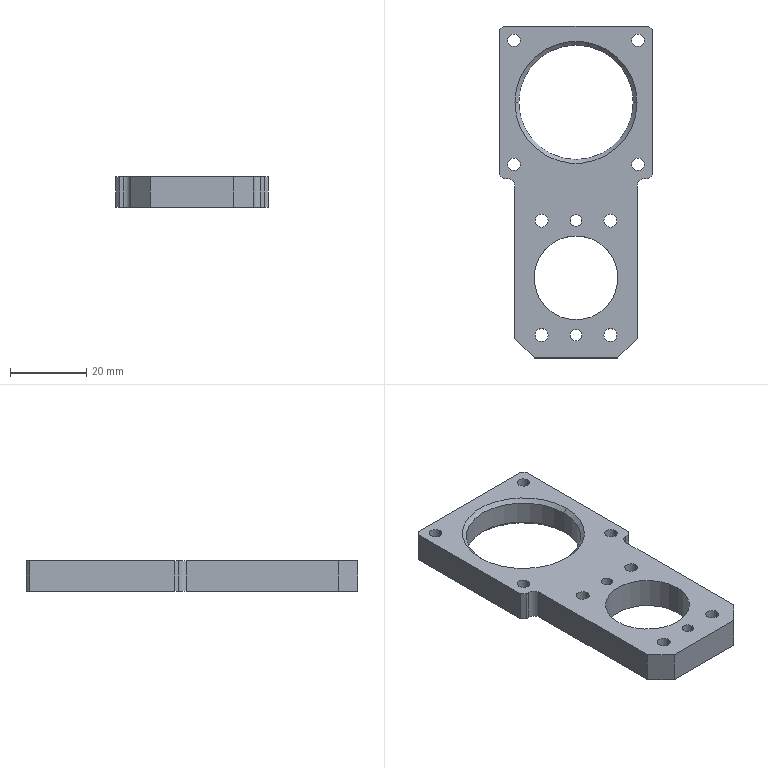Part | SolidWorks | features Chamfer 2, HoleWzd 2, Extrusion 1, Fillet 1, ICE 1 | 1 solid | 46 faces | box 40 x 87 x 8 mm | volume 15160 mm3 | cylinder 26 | plane 16 | cone 4 | commonest cylinder face diameters 3.3 x8 3.4 x8 3 x4 4 x2 22 x2 30 x2
STEP:
#1=CARTESIAN_POINT('',(-15.,23.5,3.));
#2=VERTEX_POINT('',#1);
#3=CARTESIAN_POINT('',(15.,23.5,3.));
#4=VERTEX_POINT('',#3);
#5=CARTESIAN_POINT('',(0.,23.5,3.));
#6=DIRECTION('',(0.,0.,1.));
#7=DIRECTION('',(1.,0.,0.));
#8=AXIS2_PLACEMENT_3D('',#5,#6,#7);
#9=CIRCLE('',#8,15.);
#10=EDGE_CURVE('',#2,#4,#9,.T.);
#11=ORIENTED_EDGE('',*,*,#10,.F.);
#12=CARTESIAN_POINT('',(-16.,23.5,4.));
#13=VERTEX_POINT('',#12);
#14=CARTESIAN_POINT('',(-15.,23.5,3.));
#15=DIRECTION('',(-0.7071,0.,0.7071));
#16=VECTOR('',#15,1000.);
#17=LINE('',#14,#16);
#18=EDGE_CURVE('',#2,#13,#17,.T.);
#19=ORIENTED_EDGE('',*,*,#18,.T.);
#20=CARTESIAN_POINT('',(16.,23.5,4.));
#21=VERTEX_POINT('',#20);
#22=CARTESIAN_POINT('',(0.,23.5,4.));
#23=DIRECTION('',(0.,0.,-1.));
#24=DIRECTION('',(1.,0.,0.));
#25=AXIS2_PLACEMENT_3D('',#22,#23,#24);
#26=CIRCLE('',#25,16.);
#27=EDGE_CURVE('',#21,#13,#26,.T.);
#28=ORIENTED_EDGE('',*,*,#27,.F.);
#29=CARTESIAN_POINT('',(15.,23.5,3.));
#30=DIRECTION('',(0.7071,0.,0.7071));
#31=VECTOR('',#30,1000.);
#32=LINE('',#29,#31);
#33=EDGE_CURVE('',#4,#21,#32,.T.);
#34=ORIENTED_EDGE('',*,*,#33,.F.);
#35=EDGE_LOOP('',(#11,#19,#28,#34));
#36=FACE_OUTER_BOUND('',#35,.T.);
#37=CARTESIAN_POINT('',(0.,23.5,3.));
#38=DIRECTION('',(0.,0.,1.));
#39=DIRECTION('',(1.,0.,0.));
#40=AXIS2_PLACEMENT_3D('',#37,#38,#39);
#41=CONICAL_SURFACE('',#40,15.,0.7854);
#42=ADVANCED_FACE('',(#36),#41,.F.);
#43=CARTESIAN_POINT('',(15.,23.5,-3.));
#44=VERTEX_POINT('',#43);
#45=CARTESIAN_POINT('',(-15.,23.5,-3.));
#46=VERTEX_POINT('',#45);
#47=CARTESIAN_POINT('',(0.,23.5,-3.));
#48=DIRECTION('',(0.,0.,-1.));
#49=DIRECTION('',(1.,0.,0.));
#50=AXIS2_PLACEMENT_3D('',#47,#48,#49);
#51=CIRCLE('',#50,15.);
#52=EDGE_CURVE('',#44,#46,#51,.T.);
#53=ORIENTED_EDGE('',*,*,#52,.F.);
#54=CARTESIAN_POINT('',(16.,23.5,-4.));
#55=VERTEX_POINT('',#54);
#56=CARTESIAN_POINT('',(16.,23.5,-4.));
#57=DIRECTION('',(0.7071,0.,-0.7071));
#58=VECTOR('',#57,1000.);
#59=LINE('',#56,#58);
#60=EDGE_CURVE('',#44,#55,#59,.T.);
#61=ORIENTED_EDGE('',*,*,#60,.T.);
#62=CARTESIAN_POINT('',(-16.,23.5,-4.));
#63=VERTEX_POINT('',#62);
#64=CARTESIAN_POINT('',(0.,23.5,-4.));
#65=DIRECTION('',(0.,0.,1.));
#66=DIRECTION('',(1.,0.,0.));
#67=AXIS2_PLACEMENT_3D('',#64,#65,#66);
#68=CIRCLE('',#67,16.);
#69=EDGE_CURVE('',#63,#55,#68,.T.);
#70=ORIENTED_EDGE('',*,*,#69,.F.);
#71=CARTESIAN_POINT('',(-16.,23.5,-4.));
#72=DIRECTION('',(-0.7071,0.,-0.7071));
#73=VECTOR('',#72,1000.);
#74=LINE('',#71,#73);
#75=EDGE_CURVE('',#46,#63,#74,.T.);
#76=ORIENTED_EDGE('',*,*,#75,.F.);
#77=EDGE_LOOP('',(#53,#61,#70,#76));
#78=FACE_OUTER_BOUND('',#77,.T.);
#79=CARTESIAN_POINT('',(0.,23.5,-4.));
#80=DIRECTION('',(0.,0.,-1.));
#81=DIRECTION('',(-1.,0.,0.));
#82=AXIS2_PLACEMENT_3D('',#79,#80,#81);
#83=CONICAL_SURFACE('',#82,16.,0.7854);
#84=ADVANCED_FACE('',(#78),#83,.F.);
#85=CARTESIAN_POINT('',(-11.,-22.5,-4.));
#86=VERTEX_POINT('',#85);
#87=CARTESIAN_POINT('',(11.,-22.5,-4.));
#88=VERTEX_POINT('',#87);
#89=CARTESIAN_POINT('',(0.,-22.5,-4.));
#90=DIRECTION('',(0.,0.,1.));
#91=DIRECTION('',(1.,0.,0.));
#92=AXIS2_PLACEMENT_3D('',#89,#90,#91);
#93=CIRCLE('',#92,11.);
#94=EDGE_CURVE('',#86,#88,#93,.T.);
#95=ORIENTED_EDGE('',*,*,#94,.F.);
#96=CARTESIAN_POINT('',(-11.,-22.5,4.));
#97=VERTEX_POINT('',#96);
#98=CARTESIAN_POINT('',(-11.,-22.5,-4.));
#99=DIRECTION('',(0.,0.,1.));
#100=VECTOR('',#99,1000.);
#101=LINE('',#98,#100);
#102=EDGE_CURVE('',#86,#97,#101,.T.);
#103=ORIENTED_EDGE('',*,*,#102,.T.);
#104=CARTESIAN_POINT('',(11.,-22.5,4.));
#105=VERTEX_POINT('',#104);
#106=CARTESIAN_POINT('',(0.,-22.5,4.));
#107=DIRECTION('',(0.,0.,1.));
#108=DIRECTION('',(1.,0.,0.));
#109=AXIS2_PLACEMENT_3D('',#106,#107,#108);
#110=CIRCLE('',#109,11.);
#111=EDGE_CURVE('',#97,#105,#110,.T.);
#112=ORIENTED_EDGE('',*,*,#111,.T.);
#113=CARTESIAN_POINT('',(11.,-22.5,-4.));
#114=DIRECTION('',(0.,0.,1.));
#115=VECTOR('',#114,1000.);
#116=LINE('',#113,#115);
#117=EDGE_CURVE('',#88,#105,#116,.T.);
#118=ORIENTED_EDGE('',*,*,#117,.F.);
#119=EDGE_LOOP('',(#95,#103,#112,#118));
#120=FACE_OUTER_BOUND('',#119,.T.);
#121=CARTESIAN_POINT('',(0.,-22.5,-4.));
#122=DIRECTION('',(0.,0.,1.));
#123=DIRECTION('',(1.,0.,0.));
#124=AXIS2_PLACEMENT_3D('',#121,#122,#123);
#125=CYLINDRICAL_SURFACE('',#124,11.);
#126=ADVANCED_FACE('',(#120),#125,.F.);
#127=CARTESIAN_POINT('',(-1.5,-37.5,-4.));
#128=VERTEX_POINT('',#127);
#129=CARTESIAN_POINT('',(1.5,-37.5,-4.));
#130=VERTEX_POINT('',#129);
#131=CARTESIAN_POINT('',(0.,-37.5,-4.));
#132=DIRECTION('',(0.,0.,1.));
#133=DIRECTION('',(1.,0.,0.));
#134=AXIS2_PLACEMENT_3D('',#131,#132,#133);
#135=CIRCLE('',#134,1.5);
#136=EDGE_CURVE('',#128,#130,#135,.T.);
#137=ORIENTED_EDGE('',*,*,#136,.F.);
#138=CARTESIAN_POINT('',(-1.5,-37.5,4.));
#139=VERTEX_POINT('',#138);
#140=CARTESIAN_POINT('',(-1.5,-37.5,-4.));
#141=DIRECTION('',(0.,0.,1.));
#142=VECTOR('',#141,1000.);
#143=LINE('',#140,#142);
#144=EDGE_CURVE('',#128,#139,#143,.T.);
#145=ORIENTED_EDGE('',*,*,#144,.T.);
#146=CARTESIAN_POINT('',(1.5,-37.5,4.));
#147=VERTEX_POINT('',#146);
#148=CARTESIAN_POINT('',(0.,-37.5,4.));
#149=DIRECTION('',(0.,0.,1.));
#150=DIRECTION('',(1.,0.,0.));
#151=AXIS2_PLACEMENT_3D('',#148,#149,#150);
#152=CIRCLE('',#151,1.5);
#153=EDGE_CURVE('',#139,#147,#152,.T.);
#154=ORIENTED_EDGE('',*,*,#153,.T.);
#155=CARTESIAN_POINT('',(1.5,-37.5,-4.));
#156=DIRECTION('',(0.,0.,1.));
#157=VECTOR('',#156,1000.);
#158=LINE('',#155,#157);
#159=EDGE_CURVE('',#130,#147,#158,.T.);
#160=ORIENTED_EDGE('',*,*,#159,.F.);
#161=EDGE_LOOP('',(#137,#145,#154,#160));
#162=FACE_OUTER_BOUND('',#161,.T.);
#163=CARTESIAN_POINT('',(0.,-37.5,-4.));
#164=DIRECTION('',(0.,0.,1.));
#165=DIRECTION('',(1.,0.,0.));
#166=AXIS2_PLACEMENT_3D('',#163,#164,#165);
#167=CYLINDRICAL_SURFACE('',#166,1.5);
#168=ADVANCED_FACE('',(#162),#167,.F.);
#169=CARTESIAN_POINT('',(-1.5,-7.5,-4.));
#170=VERTEX_POINT('',#169);
#171=CARTESIAN_POINT('',(1.5,-7.5,-4.));
#172=VERTEX_POINT('',#171);
#173=CARTESIAN_POINT('',(0.,-7.5,-4.));
#174=DIRECTION('',(0.,0.,1.));
#175=DIRECTION('',(1.,0.,0.));
#176=AXIS2_PLACEMENT_3D('',#173,#174,#175);
#177=CIRCLE('',#176,1.5);
#178=EDGE_CURVE('',#170,#172,#177,.T.);
#179=ORIENTED_EDGE('',*,*,#178,.F.);
#180=CARTESIAN_POINT('',(-1.5,-7.5,4.));
#181=VERTEX_POINT('',#180);
#182=CARTESIAN_POINT('',(-1.5,-7.5,-4.));
#183=DIRECTION('',(0.,0.,1.));
#184=VECTOR('',#183,1000.);
#185=LINE('',#182,#184);
#186=EDGE_CURVE('',#170,#181,#185,.T.);
#187=ORIENTED_EDGE('',*,*,#186,.T.);
#188=CARTESIAN_POINT('',(1.5,-7.5,4.));
#189=VERTEX_POINT('',#188);
#190=CARTESIAN_POINT('',(0.,-7.5,4.));
#191=DIRECTION('',(0.,0.,1.));
#192=DIRECTION('',(1.,0.,0.));
#193=AXIS2_PLACEMENT_3D('',#190,#191,#192);
#194=CIRCLE('',#193,1.5);
#195=EDGE_CURVE('',#181,#189,#194,.T.);
#196=ORIENTED_EDGE('',*,*,#195,.T.);
#197=CARTESIAN_POINT('',(1.5,-7.5,-4.));
#198=DIRECTION('',(0.,0.,1.));
#199=VECTOR('',#198,1000.);
#200=LINE('',#197,#199);
#201=EDGE_CURVE('',#172,#189,#200,.T.);
#202=ORIENTED_EDGE('',*,*,#201,.F.);
#203=EDGE_LOOP('',(#179,#187,#196,#202));
#204=FACE_OUTER_BOUND('',#203,.T.);
#205=CARTESIAN_POINT('',(0.,-7.5,-4.));
#206=DIRECTION('',(0.,0.,1.));
#207=DIRECTION('',(1.,0.,0.));
#208=AXIS2_PLACEMENT_3D('',#205,#206,#207);
#209=CYLINDRICAL_SURFACE('',#208,1.5);
#210=ADVANCED_FACE('',(#204),#209,.F.);
#211=ORIENTED_EDGE('',*,*,#52,.T.);
#212=CARTESIAN_POINT('',(-15.,23.5,-4.));
#213=DIRECTION('',(0.,0.,1.));
#214=VECTOR('',#213,1000.);
#215=LINE('',#212,#214);
#216=EDGE_CURVE('',#46,#2,#215,.T.);
#217=ORIENTED_EDGE('',*,*,#216,.T.);
#218=ORIENTED_EDGE('',*,*,#10,.T.);
#219=CARTESIAN_POINT('',(15.,23.5,-4.));
#220=DIRECTION('',(0.,0.,1.));
#221=VECTOR('',#220,1000.);
#222=LINE('',#219,#221);
#223=EDGE_CURVE('',#44,#4,#222,.T.);
#224=ORIENTED_EDGE('',*,*,#223,.F.);
#225=EDGE_LOOP('',(#211,#217,#218,#224));
#226=FACE_OUTER_BOUND('',#225,.T.);
#227=CARTESIAN_POINT('',(0.,23.5,-4.));
#228=DIRECTION('',(0.,0.,1.));
#229=DIRECTION('',(1.,0.,0.));
#230=AXIS2_PLACEMENT_3D('',#227,#228,#229);
#231=CYLINDRICAL_SURFACE('',#230,15.);
#232=ADVANCED_FACE('',(#226),#231,.F.);
#233=CARTESIAN_POINT('',(-10.7,-7.5,-4.));
#234=VERTEX_POINT('',#233);
#235=CARTESIAN_POINT('',(-7.3,-7.5,-4.));
#236=VERTEX_POINT('',#235);
#237=CARTESIAN_POINT('',(-9.,-7.5,-4.));
#238=DIRECTION('',(0.,0.,1.));
#239=DIRECTION('',(1.,0.,0.));
#240=AXIS2_PLACEMENT_3D('',#237,#238,#239);
#241=CIRCLE('',#240,1.7);
#242=EDGE_CURVE('',#234,#236,#241,.T.);
#243=ORIENTED_EDGE('',*,*,#242,.F.);
#244=CARTESIAN_POINT('',(-10.7,-7.5,4.));
#245=VERTEX_POINT('',#244);
#246=CARTESIAN_POINT('',(-10.7,-7.5,4.));
#247=DIRECTION('',(0.,0.,1.));
#248=VECTOR('',#247,1000.);
#249=LINE('',#246,#248);
#250=EDGE_CURVE('',#234,#245,#249,.T.);
#251=ORIENTED_EDGE('',*,*,#250,.T.);
#252=CARTESIAN_POINT('',(-7.3,-7.5,4.));
#253=VERTEX_POINT('',#252);
#254=CARTESIAN_POINT('',(-9.,-7.5,4.));
#255=DIRECTION('',(0.,0.,1.));
#256=DIRECTION('',(1.,0.,0.));
#257=AXIS2_PLACEMENT_3D('',#254,#255,#256);
#258=CIRCLE('',#257,1.7);
#259=EDGE_CURVE('',#245,#253,#258,.T.);
#260=ORIENTED_EDGE('',*,*,#259,.T.);
#261=CARTESIAN_POINT('',(-7.3,-7.5,4.));
#262=DIRECTION('',(0.,0.,1.));
#263=VECTOR('',#262,1000.);
#264=LINE('',#261,#263);
#265=EDGE_CURVE('',#236,#253,#264,.T.);
#266=ORIENTED_EDGE('',*,*,#265,.F.);
#267=EDGE_LOOP('',(#243,#251,#260,#266));
#268=FACE_OUTER_BOUND('',#267,.T.);
#269=CARTESIAN_POINT('',(-9.,-7.5,4.));
#270=DIRECTION('',(0.,0.,1.));
#271=DIRECTION('',(1.,0.,0.));
#272=AXIS2_PLACEMENT_3D('',#269,#270,#271);
#273=CYLINDRICAL_SURFACE('',#272,1.7);
#274=ADVANCED_FACE('',(#268),#273,.F.);
#275=CARTESIAN_POINT('',(7.3,-7.5,-4.));
#276=VERTEX_POINT('',#275);
#277=CARTESIAN_POINT('',(10.7,-7.5,-4.));
#278=VERTEX_POINT('',#277);
#279=CARTESIAN_POINT('',(9.,-7.5,-4.));
#280=DIRECTION('',(0.,0.,1.));
#281=DIRECTION('',(1.,0.,0.));
#282=AXIS2_PLACEMENT_3D('',#279,#280,#281);
#283=CIRCLE('',#282,1.7);
#284=EDGE_CURVE('',#276,#278,#283,.T.);
#285=ORIENTED_EDGE('',*,*,#284,.F.);
#286=CARTESIAN_POINT('',(7.3,-7.5,4.));
#287=VERTEX_POINT('',#286);
#288=CARTESIAN_POINT('',(7.3,-7.5,4.));
#289=DIRECTION('',(0.,0.,1.));
#290=VECTOR('',#289,1000.);
#291=LINE('',#288,#290);
#292=EDGE_CURVE('',#276,#287,#291,.T.);
#293=ORIENTED_EDGE('',*,*,#292,.T.);
#294=CARTESIAN_POINT('',(10.7,-7.5,4.));
#295=VERTEX_POINT('',#294);
#296=CARTESIAN_POINT('',(9.,-7.5,4.));
#297=DIRECTION('',(0.,0.,1.));
#298=DIRECTION('',(1.,0.,0.));
#299=AXIS2_PLACEMENT_3D('',#296,#297,#298);
#300=CIRCLE('',#299,1.7);
#301=EDGE_CURVE('',#287,#295,#300,.T.);
#302=ORIENTED_EDGE('',*,*,#301,.T.);
#303=CARTESIAN_POINT('',(10.7,-7.5,4.));
#304=DIRECTION('',(0.,0.,1.));
#305=VECTOR('',#304,1000.);
#306=LINE('',#303,#305);
#307=EDGE_CURVE('',#278,#295,#306,.T.);
#308=ORIENTED_EDGE('',*,*,#307,.F.);
#309=EDGE_LOOP('',(#285,#293,#302,#308));
#310=FACE_OUTER_BOUND('',#309,.T.);
#311=CARTESIAN_POINT('',(9.,-7.5,4.));
#312=DIRECTION('',(0.,0.,1.));
#313=DIRECTION('',(1.,0.,0.));
#314=AXIS2_PLACEMENT_3D('',#311,#312,#313);
#315=CYLINDRICAL_SURFACE('',#314,1.7);
#316=ADVANCED_FACE('',(#310),#315,.F.);
#317=CARTESIAN_POINT('',(7.3,-37.5,-4.));
#318=VERTEX_POINT('',#317);
#319=CARTESIAN_POINT('',(10.7,-37.5,-4.));
#320=VERTEX_POINT('',#319);
#321=CARTESIAN_POINT('',(9.,-37.5,-4.));
#322=DIRECTION('',(0.,0.,1.));
#323=DIRECTION('',(1.,0.,0.));
#324=AXIS2_PLACEMENT_3D('',#321,#322,#323);
#325=CIRCLE('',#324,1.7);
#326=EDGE_CURVE('',#318,#320,#325,.T.);
#327=ORIENTED_EDGE('',*,*,#326,.F.);
#328=CARTESIAN_POINT('',(7.3,-37.5,4.));
#329=VERTEX_POINT('',#328);
#330=CARTESIAN_POINT('',(7.3,-37.5,4.));
#331=DIRECTION('',(0.,0.,1.));
#332=VECTOR('',#331,1000.);
#333=LINE('',#330,#332);
#334=EDGE_CURVE('',#318,#329,#333,.T.);
#335=ORIENTED_EDGE('',*,*,#334,.T.);
#336=CARTESIAN_POINT('',(10.7,-37.5,4.));
#337=VERTEX_POINT('',#336);
#338=CARTESIAN_POINT('',(9.,-37.5,4.));
#339=DIRECTION('',(0.,0.,1.));
#340=DIRECTION('',(1.,0.,0.));
#341=AXIS2_PLACEMENT_3D('',#338,#339,#340);
#342=CIRCLE('',#341,1.7);
#343=EDGE_CURVE('',#329,#337,#342,.T.);
#344=ORIENTED_EDGE('',*,*,#343,.T.);
#345=CARTESIAN_POINT('',(10.7,-37.5,4.));
#346=DIRECTION('',(0.,0.,1.));
#347=VECTOR('',#346,1000.);
#348=LINE('',#345,#347);
#349=EDGE_CURVE('',#320,#337,#348,.T.);
#350=ORIENTED_EDGE('',*,*,#349,.F.);
#351=EDGE_LOOP('',(#327,#335,#344,#350));
#352=FACE_OUTER_BOUND('',#351,.T.);
#353=CARTESIAN_POINT('',(9.,-37.5,4.));
#354=DIRECTION('',(0.,0.,1.));
#355=DIRECTION('',(1.,0.,0.));
#356=AXIS2_PLACEMENT_3D('',#353,#354,#355);
#357=CYLINDRICAL_SURFACE('',#356,1.7);
#358=ADVANCED_FACE('',(#352),#357,.F.);
#359=CARTESIAN_POINT('',(-10.7,-37.5,-4.));
#360=VERTEX_POINT('',#359);
#361=CARTESIAN_POINT('',(-7.3,-37.5,-4.));
#362=VERTEX_POINT('',#361);
#363=CARTESIAN_POINT('',(-9.,-37.5,-4.));
#364=DIRECTION('',(0.,0.,1.));
#365=DIRECTION('',(1.,0.,0.));
#366=AXIS2_PLACEMENT_3D('',#363,#364,#365);
#367=CIRCLE('',#366,1.7);
#368=EDGE_CURVE('',#360,#362,#367,.T.);
#369=ORIENTED_EDGE('',*,*,#368,.F.);
#370=CARTESIAN_POINT('',(-10.7,-37.5,4.));
#371=VERTEX_POINT('',#370);
#372=CARTESIAN_POINT('',(-10.7,-37.5,4.));
#373=DIRECTION('',(0.,0.,1.));
#374=VECTOR('',#373,1000.);
#375=LINE('',#372,#374);
#376=EDGE_CURVE('',#360,#371,#375,.T.);
#377=ORIENTED_EDGE('',*,*,#376,.T.);
#378=CARTESIAN_POINT('',(-7.3,-37.5,4.));
#379=VERTEX_POINT('',#378);
#380=CARTESIAN_POINT('',(-9.,-37.5,4.));
#381=DIRECTION('',(0.,0.,1.));
#382=DIRECTION('',(1.,0.,0.));
#383=AXIS2_PLACEMENT_3D('',#380,#381,#382);
#384=CIRCLE('',#383,1.7);
#385=EDGE_CURVE('',#371,#379,#384,.T.);
#386=ORIENTED_EDGE('',*,*,#385,.T.);
#387=CARTESIAN_POINT('',(-7.3,-37.5,4.));
#388=DIRECTION('',(0.,0.,1.));
#389=VECTOR('',#388,1000.);
#390=LINE('',#387,#389);
#391=EDGE_CURVE('',#362,#379,#390,.T.);
#392=ORIENTED_EDGE('',*,*,#391,.F.);
#393=EDGE_LOOP('',(#369,#377,#386,#392));
#394=FACE_OUTER_BOUND('',#393,.T.);
#395=CARTESIAN_POINT('',(-9.,-37.5,4.));
#396=DIRECTION('',(0.,0.,1.));
#397=DIRECTION('',(1.,0.,0.));
#398=AXIS2_PLACEMENT_3D('',#395,#396,#397);
#399=CYLINDRICAL_SURFACE('',#398,1.7);
#400=ADVANCED_FACE('',(#394),#399,.F.);
#401=CARTESIAN_POINT('',(-17.913,39.763,-4.));
#402=VERTEX_POINT('',#401);
#403=CARTESIAN_POINT('',(-14.613,39.763,-4.));
#404=VERTEX_POINT('',#403);
#405=CARTESIAN_POINT('',(-16.263,39.763,-4.));
#406=DIRECTION('',(0.,0.,1.));
#407=DIRECTION('',(1.,0.,0.));
#408=AXIS2_PLACEMENT_3D('',#405,#406,#407);
#409=CIRCLE('',#408,1.65);
#410=EDGE_CURVE('',#402,#404,#409,.T.);
#411=ORIENTED_EDGE('',*,*,#410,.F.);
#412=CARTESIAN_POINT('',(-17.913,39.763,4.));
#413=VERTEX_POINT('',#412);
#414=CARTESIAN_POINT('',(-17.913,39.763,4.));
#415=DIRECTION('',(0.,0.,1.));
#416=VECTOR('',#415,1000.);
#417=LINE('',#414,#416);
#418=EDGE_CURVE('',#402,#413,#417,.T.);
#419=ORIENTED_EDGE('',*,*,#418,.T.);
#420=CARTESIAN_POINT('',(-14.613,39.763,4.));
#421=VERTEX_POINT('',#420);
#422=CARTESIAN_POINT('',(-16.263,39.763,4.));
#423=DIRECTION('',(0.,0.,1.));
#424=DIRECTION('',(1.,0.,0.));
#425=AXIS2_PLACEMENT_3D('',#422,#423,#424);
#426=CIRCLE('',#425,1.65);
#427=EDGE_CURVE('',#413,#421,#426,.T.);
#428=ORIENTED_EDGE('',*,*,#427,.T.);
#429=CARTESIAN_POINT('',(-14.613,39.763,4.));
#430=DIRECTION('',(0.,0.,1.));
#431=VECTOR('',#430,1000.);
#432=LINE('',#429,#431);
#433=EDGE_CURVE('',#404,#421,#432,.T.);
#434=ORIENTED_EDGE('',*,*,#433,.F.);
#435=EDGE_LOOP('',(#411,#419,#428,#434));
#436=FACE_OUTER_BOUND('',#435,.T.);
#437=CARTESIAN_POINT('',(-16.263,39.763,4.));
#438=DIRECTION('',(0.,0.,1.));
#439=DIRECTION('',(1.,0.,0.));
#440=AXIS2_PLACEMENT_3D('',#437,#438,#439);
#441=CYLINDRICAL_SURFACE('',#440,1.65);
#442=ADVANCED_FACE('',(#436),#441,.F.);
#443=CARTESIAN_POINT('',(14.613,39.763,-4.));
#444=VERTEX_POINT('',#443);
#445=CARTESIAN_POINT('',(17.913,39.763,-4.));
#446=VERTEX_POINT('',#445);
#447=CARTESIAN_POINT('',(16.263,39.763,-4.));
#448=DIRECTION('',(0.,0.,1.));
#449=DIRECTION('',(1.,0.,0.));
#450=AXIS2_PLACEMENT_3D('',#447,#448,#449);
#451=CIRCLE('',#450,1.65);
#452=EDGE_CURVE('',#444,#446,#451,.T.);
#453=ORIENTED_EDGE('',*,*,#452,.F.);
#454=CARTESIAN_POINT('',(14.613,39.763,4.));
#455=VERTEX_POINT('',#454);
#456=CARTESIAN_POINT('',(14.613,39.763,4.));
#457=DIRECTION('',(0.,0.,1.));
#458=VECTOR('',#457,1000.);
#459=LINE('',#456,#458);
#460=EDGE_CURVE('',#444,#455,#459,.T.);
#461=ORIENTED_EDGE('',*,*,#460,.T.);
#462=CARTESIAN_POINT('',(17.913,39.763,4.));
#463=VERTEX_POINT('',#462);
#464=CARTESIAN_POINT('',(16.263,39.763,4.));
#465=DIRECTION('',(0.,0.,1.));
#466=DIRECTION('',(1.,0.,0.));
#467=AXIS2_PLACEMENT_3D('',#464,#465,#466);
#468=CIRCLE('',#467,1.65);
#469=EDGE_CURVE('',#455,#463,#468,.T.);
#470=ORIENTED_EDGE('',*,*,#469,.T.);
#471=CARTESIAN_POINT('',(17.913,39.763,4.));
#472=DIRECTION('',(0.,0.,1.));
#473=VECTOR('',#472,1000.);
#474=LINE('',#471,#473);
#475=EDGE_CURVE('',#446,#463,#474,.T.);
#476=ORIENTED_EDGE('',*,*,#475,.F.);
#477=EDGE_LOOP('',(#453,#461,#470,#476));
#478=FACE_OUTER_BOUND('',#477,.T.);
#479=CARTESIAN_POINT('',(16.263,39.763,4.));
#480=DIRECTION('',(0.,0.,1.));
#481=DIRECTION('',(1.,0.,0.));
#482=AXIS2_PLACEMENT_3D('',#479,#480,#481);
#483=CYLINDRICAL_SURFACE('',#482,1.65);
#484=ADVANCED_FACE('',(#478),#483,.F.);
#485=CARTESIAN_POINT('',(14.613,7.237,-4.));
#486=VERTEX_POINT('',#485);
#487=CARTESIAN_POINT('',(17.913,7.237,-4.));
#488=VERTEX_POINT('',#487);
#489=CARTESIAN_POINT('',(16.263,7.237,-4.));
#490=DIRECTION('',(0.,0.,1.));
#491=DIRECTION('',(1.,0.,0.));
#492=AXIS2_PLACEMENT_3D('',#489,#490,#491);
#493=CIRCLE('',#492,1.65);
#494=EDGE_CURVE('',#486,#488,#493,.T.);
#495=ORIENTED_EDGE('',*,*,#494,.F.);
#496=CARTESIAN_POINT('',(14.613,7.237,4.));
#497=VERTEX_POINT('',#496);
#498=CARTESIAN_POINT('',(14.613,7.237,4.));
#499=DIRECTION('',(0.,0.,1.));
#500=VECTOR('',#499,1000.);
#501=LINE('',#498,#500);
#502=EDGE_CURVE('',#486,#497,#501,.T.);
#503=ORIENTED_EDGE('',*,*,#502,.T.);
#504=CARTESIAN_POINT('',(17.913,7.237,4.));
#505=VERTEX_POINT('',#504);
#506=CARTESIAN_POINT('',(16.263,7.237,4.));
#507=DIRECTION('',(0.,0.,1.));
#508=DIRECTION('',(1.,0.,0.));
#509=AXIS2_PLACEMENT_3D('',#506,#507,#508);
#510=CIRCLE('',#509,1.65);
#511=EDGE_CURVE('',#497,#505,#510,.T.);
#512=ORIENTED_EDGE('',*,*,#511,.T.);
#513=CARTESIAN_POINT('',(17.913,7.237,4.));
#514=DIRECTION('',(0.,0.,1.));
#515=VECTOR('',#514,1000.);
#516=LINE('',#513,#515);
#517=EDGE_CURVE('',#488,#505,#516,.T.);
#518=ORIENTED_EDGE('',*,*,#517,.F.);
#519=EDGE_LOOP('',(#495,#503,#512,#518));
#520=FACE_OUTER_BOUND('',#519,.T.);
#521=CARTESIAN_POINT('',(16.263,7.237,4.));
#522=DIRECTION('',(0.,0.,1.));
#523=DIRECTION('',(1.,0.,0.));
#524=AXIS2_PLACEMENT_3D('',#521,#522,#523);
#525=CYLINDRICAL_SURFACE('',#524,1.65);
#526=ADVANCED_FACE('',(#520),#525,.F.);
#527=CARTESIAN_POINT('',(-17.913,7.237,-4.));
#528=VERTEX_POINT('',#527);
#529=CARTESIAN_POINT('',(-14.613,7.237,-4.));
#530=VERTEX_POINT('',#529);
#531=CARTESIAN_POINT('',(-16.263,7.237,-4.));
#532=DIRECTION('',(0.,0.,1.));
#533=DIRECTION('',(1.,0.,0.));
#534=AXIS2_PLACEMENT_3D('',#531,#532,#533);
#535=CIRCLE('',#534,1.65);
#536=EDGE_CURVE('',#528,#530,#535,.T.);
#537=ORIENTED_EDGE('',*,*,#536,.F.);
#538=CARTESIAN_POINT('',(-17.913,7.237,4.));
#539=VERTEX_POINT('',#538);
#540=CARTESIAN_POINT('',(-17.913,7.237,4.));
#541=DIRECTION('',(0.,0.,1.));
#542=VECTOR('',#541,1000.);
#543=LINE('',#540,#542);
#544=EDGE_CURVE('',#528,#539,#543,.T.);
#545=ORIENTED_EDGE('',*,*,#544,.T.);
#546=CARTESIAN_POINT('',(-14.613,7.237,4.));
#547=VERTEX_POINT('',#546);
#548=CARTESIAN_POINT('',(-16.263,7.237,4.));
#549=DIRECTION('',(0.,0.,1.));
#550=DIRECTION('',(1.,0.,0.));
#551=AXIS2_PLACEMENT_3D('',#548,#549,#550);
#552=CIRCLE('',#551,1.65);
#553=EDGE_CURVE('',#539,#547,#552,.T.);
#554=ORIENTED_EDGE('',*,*,#553,.T.);
#555=CARTESIAN_POINT('',(-14.613,7.237,4.));
#556=DIRECTION('',(0.,0.,1.));
#557=VECTOR('',#556,1000.);
#558=LINE('',#555,#557);
#559=EDGE_CURVE('',#530,#547,#558,.T.);
#560=ORIENTED_EDGE('',*,*,#559,.F.);
#561=EDGE_LOOP('',(#537,#545,#554,#560));
#562=FACE_OUTER_BOUND('',#561,.T.);
#563=CARTESIAN_POINT('',(-16.263,7.237,4.));
#564=DIRECTION('',(0.,0.,1.));
#565=DIRECTION('',(1.,0.,0.));
#566=AXIS2_PLACEMENT_3D('',#563,#564,#565);
#567=CYLINDRICAL_SURFACE('',#566,1.65);
#568=ADVANCED_FACE('',(#562),#567,.F.);
#569=CARTESIAN_POINT('',(-16.,-38.5,4.));
#570=VERTEX_POINT('',#569);
#571=CARTESIAN_POINT('',(-16.,1.5,4.));
#572=VERTEX_POINT('',#571);
#573=CARTESIAN_POINT('',(-16.,0.,4.));
#574=DIRECTION('',(0.,1.,0.));
#575=VECTOR('',#574,1000.);
#576=LINE('',#573,#575);
#577=EDGE_CURVE('',#570,#572,#576,.T.);
#578=ORIENTED_EDGE('',*,*,#577,.T.);
#579=CARTESIAN_POINT('',(-16.,1.5,-4.));
#580=VERTEX_POINT('',#579);
#581=CARTESIAN_POINT('',(-16.,1.5,4.));
#582=DIRECTION('',(0.,0.,-1.));
#583=VECTOR('',#582,1000.);
#584=LINE('',#581,#583);
#585=EDGE_CURVE('',#572,#580,#584,.T.);
#586=ORIENTED_EDGE('',*,*,#585,.T.);
#587=CARTESIAN_POINT('',(-16.,-38.5,-4.));
#588=VERTEX_POINT('',#587);
#589=CARTESIAN_POINT('',(-16.,0.,-4.));
#590=DIRECTION('',(0.,1.,0.));
#591=VECTOR('',#590,1000.);
#592=LINE('',#589,#591);
#593=EDGE_CURVE('',#588,#580,#592,.T.);
#594=ORIENTED_EDGE('',*,*,#593,.F.);
#595=CARTESIAN_POINT('',(-16.,-38.5,4.));
#596=DIRECTION('',(0.,0.,1.));
#597=VECTOR('',#596,1000.);
#598=LINE('',#595,#597);
#599=EDGE_CURVE('',#588,#570,#598,.T.);
#600=ORIENTED_EDGE('',*,*,#599,.T.);
#601=EDGE_LOOP('',(#578,#586,#594,#600));
#602=FACE_OUTER_BOUND('',#601,.T.);
#603=CARTESIAN_POINT('',(-16.,0.,4.));
#604=DIRECTION('',(-1.,0.,0.));
#605=DIRECTION('',(0.,-1.,0.));
#606=AXIS2_PLACEMENT_3D('',#603,#604,#605);
#607=PLANE('',#606);
#608=ADVANCED_FACE('',(#602),#607,.T.);
#609=CARTESIAN_POINT('',(-11.,-43.5,4.));
#610=VERTEX_POINT('',#609);
#611=CARTESIAN_POINT('',(11.,-43.5,4.));
#612=VERTEX_POINT('',#611);
#613=CARTESIAN_POINT('',(0.,-43.5,4.));
#614=DIRECTION('',(1.,0.,0.));
#615=VECTOR('',#614,1000.);
#616=LINE('',#613,#615);
#617=EDGE_CURVE('',#610,#612,#616,.T.);
#618=ORIENTED_EDGE('',*,*,#617,.F.);
#619=CARTESIAN_POINT('',(-11.,-43.5,-4.));
#620=VERTEX_POINT('',#619);
#621=CARTESIAN_POINT('',(-11.,-43.5,-4.));
#622=DIRECTION('',(0.,0.,-1.));
#623=VECTOR('',#622,1000.);
#624=LINE('',#621,#623);
#625=EDGE_CURVE('',#610,#620,#624,.T.);
#626=ORIENTED_EDGE('',*,*,#625,.T.);
#627=CARTESIAN_POINT('',(11.,-43.5,-4.));
#628=VERTEX_POINT('',#627);
#629=CARTESIAN_POINT('',(0.,-43.5,-4.));
#630=DIRECTION('',(1.,0.,0.));
#631=VECTOR('',#630,1000.);
#632=LINE('',#629,#631);
#633=EDGE_CURVE('',#620,#628,#632,.T.);
#634=ORIENTED_EDGE('',*,*,#633,.T.);
#635=CARTESIAN_POINT('',(11.,-43.5,4.));
#636=DIRECTION('',(0.,0.,1.));
#637=VECTOR('',#636,1000.);
#638=LINE('',#635,#637);
#639=EDGE_CURVE('',#628,#612,#638,.T.);
#640=ORIENTED_EDGE('',*,*,#639,.T.);
#641=EDGE_LOOP('',(#618,#626,#634,#640));
#642=FACE_OUTER_BOUND('',#641,.T.);
#643=CARTESIAN_POINT('',(0.,-43.5,4.));
#644=DIRECTION('',(0.,1.,0.));
#645=DIRECTION('',(-1.,0.,0.));
#646=AXIS2_PLACEMENT_3D('',#643,#644,#645);
#647=PLANE('',#646);
#648=ADVANCED_FACE('',(#642),#647,.F.);
#649=CARTESIAN_POINT('',(16.,-38.5,-4.));
#650=VERTEX_POINT('',#649);
#651=CARTESIAN_POINT('',(16.,1.5,-4.));
#652=VERTEX_POINT('',#651);
#653=CARTESIAN_POINT('',(16.,0.,-4.));
#654=DIRECTION('',(0.,1.,0.));
#655=VECTOR('',#654,1000.);
#656=LINE('',#653,#655);
#657=EDGE_CURVE('',#650,#652,#656,.T.);
#658=ORIENTED_EDGE('',*,*,#657,.T.);
#659=CARTESIAN_POINT('',(16.,1.5,4.));
#660=VERTEX_POINT('',#659);
#661=CARTESIAN_POINT('',(16.,1.5,4.));
#662=DIRECTION('',(0.,0.,1.));
#663=VECTOR('',#662,1000.);
#664=LINE('',#661,#663);
#665=EDGE_CURVE('',#652,#660,#664,.T.);
#666=ORIENTED_EDGE('',*,*,#665,.T.);
#667=CARTESIAN_POINT('',(16.,-38.5,4.));
#668=VERTEX_POINT('',#667);
#669=CARTESIAN_POINT('',(16.,0.,4.));
#670=DIRECTION('',(0.,1.,0.));
#671=VECTOR('',#670,1000.);
#672=LINE('',#669,#671);
#673=EDGE_CURVE('',#668,#660,#672,.T.);
#674=ORIENTED_EDGE('',*,*,#673,.F.);
#675=CARTESIAN_POINT('',(16.,-38.5,4.));
#676=DIRECTION('',(0.,0.,-1.));
#677=VECTOR('',#676,1000.);
#678=LINE('',#675,#677);
#679=EDGE_CURVE('',#668,#650,#678,.T.);
#680=ORIENTED_EDGE('',*,*,#679,.T.);
#681=EDGE_LOOP('',(#658,#666,#674,#680));
#682=FACE_OUTER_BOUND('',#681,.T.);
#683=CARTESIAN_POINT('',(16.,0.,4.));
#684=DIRECTION('',(-1.,0.,0.));
#685=DIRECTION('',(0.,0.,1.));
#686=AXIS2_PLACEMENT_3D('',#683,#684,#685);
#687=PLANE('',#686);
#688=ADVANCED_FACE('',(#682),#687,.F.);
#689=CARTESIAN_POINT('',(19.,3.5,4.));
#690=VERTEX_POINT('',#689);
#691=CARTESIAN_POINT('',(18.,3.5,4.));
#692=VERTEX_POINT('',#691);
#693=CARTESIAN_POINT('',(0.,3.5,4.));
#694=DIRECTION('',(-1.,0.,0.));
#695=VECTOR('',#694,1000.);
#696=LINE('',#693,#695);
#697=EDGE_CURVE('',#690,#692,#696,.T.);
#698=ORIENTED_EDGE('',*,*,#697,.T.);
#699=CARTESIAN_POINT('',(18.,3.5,-4.));
#700=VERTEX_POINT('',#699);
#701=CARTESIAN_POINT('',(18.,3.5,4.));
#702=DIRECTION('',(0.,0.,-1.));
#703=VECTOR('',#702,1000.);
#704=LINE('',#701,#703);
#705=EDGE_CURVE('',#692,#700,#704,.T.);
#706=ORIENTED_EDGE('',*,*,#705,.T.);
#707=CARTESIAN_POINT('',(19.,3.5,-4.));
#708=VERTEX_POINT('',#707);
#709=CARTESIAN_POINT('',(0.,3.5,-4.));
#710=DIRECTION('',(-1.,0.,0.));
#711=VECTOR('',#710,1000.);
#712=LINE('',#709,#711);
#713=EDGE_CURVE('',#708,#700,#712,.T.);
#714=ORIENTED_EDGE('',*,*,#713,.F.);
#715=CARTESIAN_POINT('',(19.,3.5,4.));
#716=DIRECTION('',(0.,0.,1.));
#717=VECTOR('',#716,1000.);
#718=LINE('',#715,#717);
#719=EDGE_CURVE('',#708,#690,#718,.T.);
#720=ORIENTED_EDGE('',*,*,#719,.T.);
#721=EDGE_LOOP('',(#698,#706,#714,#720));
#722=FACE_OUTER_BOUND('',#721,.T.);
#723=CARTESIAN_POINT('',(0.,3.5,4.));
#724=DIRECTION('',(0.,-1.,0.));
#725=DIRECTION('',(1.,0.,0.));
#726=AXIS2_PLACEMENT_3D('',#723,#724,#725);
#727=PLANE('',#726);
#728=ADVANCED_FACE('',(#722),#727,.T.);
#729=CARTESIAN_POINT('',(20.,4.5,-4.));
#730=VERTEX_POINT('',#729);
#731=CARTESIAN_POINT('',(20.,42.5,-4.));
#732=VERTEX_POINT('',#731);
#733=CARTESIAN_POINT('',(20.,0.,-4.));
#734=DIRECTION('',(0.,1.,0.));
#735=VECTOR('',#734,1000.);
#736=LINE('',#733,#735);
#737=EDGE_CURVE('',#730,#732,#736,.T.);
#738=ORIENTED_EDGE('',*,*,#737,.T.);
#739=CARTESIAN_POINT('',(20.,42.5,4.));
#740=VERTEX_POINT('',#739);
#741=CARTESIAN_POINT('',(20.,42.5,4.));
#742=DIRECTION('',(0.,0.,1.));
#743=VECTOR('',#742,1000.);
#744=LINE('',#741,#743);
#745=EDGE_CURVE('',#732,#740,#744,.T.);
#746=ORIENTED_EDGE('',*,*,#745,.T.);
#747=CARTESIAN_POINT('',(20.,4.5,4.));
#748=VERTEX_POINT('',#747);
#749=CARTESIAN_POINT('',(20.,0.,4.));
#750=DIRECTION('',(0.,1.,0.));
#751=VECTOR('',#750,1000.);
#752=LINE('',#749,#751);
#753=EDGE_CURVE('',#748,#740,#752,.T.);
#754=ORIENTED_EDGE('',*,*,#753,.F.);
#755=CARTESIAN_POINT('',(20.,4.5,-4.));
#756=DIRECTION('',(0.,0.,-1.));
#757=VECTOR('',#756,1000.);
#758=LINE('',#755,#757);
#759=EDGE_CURVE('',#748,#730,#758,.T.);
#760=ORIENTED_EDGE('',*,*,#759,.T.);
#761=EDGE_LOOP('',(#738,#746,#754,#760));
#762=FACE_OUTER_BOUND('',#761,.T.);
#763=CARTESIAN_POINT('',(20.,0.,4.));
#764=DIRECTION('',(-1.,0.,0.));
#765=DIRECTION('',(0.,-1.,0.));
#766=AXIS2_PLACEMENT_3D('',#763,#764,#765);
#767=PLANE('',#766);
#768=ADVANCED_FACE('',(#762),#767,.F.);
#769=CARTESIAN_POINT('',(-19.,43.5,-4.));
#770=VERTEX_POINT('',#769);
#771=CARTESIAN_POINT('',(19.,43.5,-4.));
#772=VERTEX_POINT('',#771);
#773=CARTESIAN_POINT('',(0.,43.5,-4.));
#774=DIRECTION('',(1.,0.,0.));
#775=VECTOR('',#774,1000.);
#776=LINE('',#773,#775);
#777=EDGE_CURVE('',#770,#772,#776,.T.);
#778=ORIENTED_EDGE('',*,*,#777,.F.);
#779=CARTESIAN_POINT('',(-19.,43.5,4.));
#780=VERTEX_POINT('',#779);
#781=CARTESIAN_POINT('',(-19.,43.5,4.));
#782=DIRECTION('',(0.,0.,1.));
#783=VECTOR('',#782,1000.);
#784=LINE('',#781,#783);
#785=EDGE_CURVE('',#770,#780,#784,.T.);
#786=ORIENTED_EDGE('',*,*,#785,.T.);
#787=CARTESIAN_POINT('',(19.,43.5,4.));
#788=VERTEX_POINT('',#787);
#789=CARTESIAN_POINT('',(0.,43.5,4.));
#790=DIRECTION('',(1.,0.,0.));
#791=VECTOR('',#790,1000.);
#792=LINE('',#789,#791);
#793=EDGE_CURVE('',#780,#788,#792,.T.);
#794=ORIENTED_EDGE('',*,*,#793,.T.);
#795=CARTESIAN_POINT('',(19.,43.5,-4.));
#796=DIRECTION('',(0.,0.,-1.));
#797=VECTOR('',#796,1000.);
#798=LINE('',#795,#797);
#799=EDGE_CURVE('',#788,#772,#798,.T.);
#800=ORIENTED_EDGE('',*,*,#799,.T.);
#801=EDGE_LOOP('',(#778,#786,#794,#800));
#802=FACE_OUTER_BOUND('',#801,.T.);
#803=CARTESIAN_POINT('',(0.,43.5,4.));
#804=DIRECTION('',(0.,1.,0.));
#805=DIRECTION('',(0.,0.,1.));
#806=AXIS2_PLACEMENT_3D('',#803,#804,#805);
#807=PLANE('',#806);
#808=ADVANCED_FACE('',(#802),#807,.T.);
#809=CARTESIAN_POINT('',(-20.,4.5,4.));
#810=VERTEX_POINT('',#809);
#811=CARTESIAN_POINT('',(-20.,42.5,4.));
#812=VERTEX_POINT('',#811);
#813=CARTESIAN_POINT('',(-20.,0.,4.));
#814=DIRECTION('',(0.,1.,0.));
#815=VECTOR('',#814,1000.);
#816=LINE('',#813,#815);
#817=EDGE_CURVE('',#810,#812,#816,.T.);
#818=ORIENTED_EDGE('',*,*,#817,.T.);
#819=CARTESIAN_POINT('',(-20.,42.5,-4.));
#820=VERTEX_POINT('',#819);
#821=CARTESIAN_POINT('',(-20.,42.5,4.));
#822=DIRECTION('',(0.,0.,-1.));
#823=VECTOR('',#822,1000.);
#824=LINE('',#821,#823);
#825=EDGE_CURVE('',#812,#820,#824,.T.);
#826=ORIENTED_EDGE('',*,*,#825,.T.);
#827=CARTESIAN_POINT('',(-20.,4.5,-4.));
#828=VERTEX_POINT('',#827);
#829=CARTESIAN_POINT('',(-20.,0.,-4.));
#830=DIRECTION('',(0.,1.,0.));
#831=VECTOR('',#830,1000.);
#832=LINE('',#829,#831);
#833=EDGE_CURVE('',#828,#820,#832,.T.);
#834=ORIENTED_EDGE('',*,*,#833,.F.);
#835=CARTESIAN_POINT('',(-20.,4.5,4.));
#836=DIRECTION('',(0.,0.,1.));
#837=VECTOR('',#836,1000.);
#838=LINE('',#835,#837);
#839=EDGE_CURVE('',#828,#810,#838,.T.);
#840=ORIENTED_EDGE('',*,*,#839,.T.);
#841=EDGE_LOOP('',(#818,#826,#834,#840));
#842=FACE_OUTER_BOUND('',#841,.T.);
#843=CARTESIAN_POINT('',(-20.,0.,4.));
#844=DIRECTION('',(-1.,0.,0.));
#845=DIRECTION('',(0.,0.,1.));
#846=AXIS2_PLACEMENT_3D('',#843,#844,#845);
#847=PLANE('',#846);
#848=ADVANCED_FACE('',(#842),#847,.T.);
#849=CARTESIAN_POINT('',(-19.,3.5,-4.));
#850=VERTEX_POINT('',#849);
#851=CARTESIAN_POINT('',(-18.,3.5,-4.));
#852=VERTEX_POINT('',#851);
#853=CARTESIAN_POINT('',(0.,3.5,-4.));
#854=DIRECTION('',(1.,0.,0.));
#855=VECTOR('',#854,1000.);
#856=LINE('',#853,#855);
#857=EDGE_CURVE('',#850,#852,#856,.T.);
#858=ORIENTED_EDGE('',*,*,#857,.T.);
#859=CARTESIAN_POINT('',(-18.,3.5,4.));
#860=VERTEX_POINT('',#859);
#861=CARTESIAN_POINT('',(-18.,3.5,4.));
#862=DIRECTION('',(0.,0.,1.));
#863=VECTOR('',#862,1000.);
#864=LINE('',#861,#863);
#865=EDGE_CURVE('',#852,#860,#864,.T.);
#866=ORIENTED_EDGE('',*,*,#865,.T.);
#867=CARTESIAN_POINT('',(-19.,3.5,4.));
#868=VERTEX_POINT('',#867);
#869=CARTESIAN_POINT('',(0.,3.5,4.));
#870=DIRECTION('',(1.,0.,0.));
#871=VECTOR('',#870,1000.);
#872=LINE('',#869,#871);
#873=EDGE_CURVE('',#868,#860,#872,.T.);
#874=ORIENTED_EDGE('',*,*,#873,.F.);
#875=CARTESIAN_POINT('',(-19.,3.5,-4.));
#876=DIRECTION('',(0.,0.,-1.));
#877=VECTOR('',#876,1000.);
#878=LINE('',#875,#877);
#879=EDGE_CURVE('',#868,#850,#878,.T.);
#880=ORIENTED_EDGE('',*,*,#879,.T.);
#881=EDGE_LOOP('',(#858,#866,#874,#880));
#882=FACE_OUTER_BOUND('',#881,.T.);
#883=CARTESIAN_POINT('',(0.,3.5,4.));
#884=DIRECTION('',(0.,1.,0.));
#885=DIRECTION('',(-1.,0.,0.));
#886=AXIS2_PLACEMENT_3D('',#883,#884,#885);
#887=PLANE('',#886);
#888=ADVANCED_FACE('',(#882),#887,.F.);
#889=ORIENTED_EDGE('',*,*,#27,.T.);
#890=CARTESIAN_POINT('',(0.,23.5,4.));
#891=DIRECTION('',(0.,0.,-1.));
#892=DIRECTION('',(1.,0.,0.));
#893=AXIS2_PLACEMENT_3D('',#890,#891,#892);
#894=CIRCLE('',#893,16.);
#895=EDGE_CURVE('',#13,#21,#894,.T.);
#896=ORIENTED_EDGE('',*,*,#895,.T.);
#897=EDGE_LOOP('',(#889,#896));
#898=FACE_BOUND('',#897,.T.);
#899=CARTESIAN_POINT('',(0.,-22.5,4.));
#900=DIRECTION('',(0.,0.,1.));
#901=DIRECTION('',(1.,0.,0.));
#902=AXIS2_PLACEMENT_3D('',#899,#900,#901);
#903=CIRCLE('',#902,11.);
#904=EDGE_CURVE('',#105,#97,#903,.T.);
#905=ORIENTED_EDGE('',*,*,#904,.F.);
#906=ORIENTED_EDGE('',*,*,#111,.F.);
#907=EDGE_LOOP('',(#905,#906));
#908=FACE_BOUND('',#907,.T.);
#909=CARTESIAN_POINT('',(0.,-37.5,4.));
#910=DIRECTION('',(0.,0.,1.));
#911=DIRECTION('',(1.,0.,0.));
#912=AXIS2_PLACEMENT_3D('',#909,#910,#911);
#913=CIRCLE('',#912,1.5);
#914=EDGE_CURVE('',#147,#139,#913,.T.);
#915=ORIENTED_EDGE('',*,*,#914,.F.);
#916=ORIENTED_EDGE('',*,*,#153,.F.);
#917=EDGE_LOOP('',(#915,#916));
#918=FACE_BOUND('',#917,.T.);
#919=CARTESIAN_POINT('',(0.,-7.5,4.));
#920=DIRECTION('',(0.,0.,1.));
#921=DIRECTION('',(1.,0.,0.));
#922=AXIS2_PLACEMENT_3D('',#919,#920,#921);
#923=CIRCLE('',#922,1.5);
#924=EDGE_CURVE('',#189,#181,#923,.T.);
#925=ORIENTED_EDGE('',*,*,#924,.F.);
#926=ORIENTED_EDGE('',*,*,#195,.F.);
#927=EDGE_LOOP('',(#925,#926));
#928=FACE_BOUND('',#927,.T.);
#929=CARTESIAN_POINT('',(-9.,-7.5,4.));
#930=DIRECTION('',(0.,0.,1.));
#931=DIRECTION('',(1.,0.,0.));
#932=AXIS2_PLACEMENT_3D('',#929,#930,#931);
#933=CIRCLE('',#932,1.7);
#934=EDGE_CURVE('',#253,#245,#933,.T.);
#935=ORIENTED_EDGE('',*,*,#934,.F.);
#936=ORIENTED_EDGE('',*,*,#259,.F.);
#937=EDGE_LOOP('',(#935,#936));
#938=FACE_BOUND('',#937,.T.);
#939=CARTESIAN_POINT('',(9.,-7.5,4.));
#940=DIRECTION('',(0.,0.,1.));
#941=DIRECTION('',(1.,0.,0.));
#942=AXIS2_PLACEMENT_3D('',#939,#940,#941);
#943=CIRCLE('',#942,1.7);
#944=EDGE_CURVE('',#295,#287,#943,.T.);
#945=ORIENTED_EDGE('',*,*,#944,.F.);
#946=ORIENTED_EDGE('',*,*,#301,.F.);
#947=EDGE_LOOP('',(#945,#946));
#948=FACE_BOUND('',#947,.T.);
#949=CARTESIAN_POINT('',(9.,-37.5,4.));
#950=DIRECTION('',(0.,0.,1.));
#951=DIRECTION('',(1.,0.,0.));
#952=AXIS2_PLACEMENT_3D('',#949,#950,#951);
#953=CIRCLE('',#952,1.7);
#954=EDGE_CURVE('',#337,#329,#953,.T.);
#955=ORIENTED_EDGE('',*,*,#954,.F.);
#956=ORIENTED_EDGE('',*,*,#343,.F.);
#957=EDGE_LOOP('',(#955,#956));
#958=FACE_BOUND('',#957,.T.);
#959=CARTESIAN_POINT('',(-9.,-37.5,4.));
#960=DIRECTION('',(0.,0.,1.));
#961=DIRECTION('',(1.,0.,0.));
#962=AXIS2_PLACEMENT_3D('',#959,#960,#961);
#963=CIRCLE('',#962,1.7);
#964=EDGE_CURVE('',#379,#371,#963,.T.);
#965=ORIENTED_EDGE('',*,*,#964,.F.);
#966=ORIENTED_EDGE('',*,*,#385,.F.);
#967=EDGE_LOOP('',(#965,#966));
#968=FACE_BOUND('',#967,.T.);
#969=CARTESIAN_POINT('',(-16.263,39.763,4.));
#970=DIRECTION('',(0.,0.,1.));
#971=DIRECTION('',(1.,0.,0.));
#972=AXIS2_PLACEMENT_3D('',#969,#970,#971);
#973=CIRCLE('',#972,1.65);
#974=EDGE_CURVE('',#421,#413,#973,.T.);
#975=ORIENTED_EDGE('',*,*,#974,.F.);
#976=ORIENTED_EDGE('',*,*,#427,.F.);
#977=EDGE_LOOP('',(#975,#976));
#978=FACE_BOUND('',#977,.T.);
#979=CARTESIAN_POINT('',(16.263,39.763,4.));
#980=DIRECTION('',(0.,0.,1.));
#981=DIRECTION('',(1.,0.,0.));
#982=AXIS2_PLACEMENT_3D('',#979,#980,#981);
#983=CIRCLE('',#982,1.65);
#984=EDGE_CURVE('',#463,#455,#983,.T.);
#985=ORIENTED_EDGE('',*,*,#984,.F.);
#986=ORIENTED_EDGE('',*,*,#469,.F.);
#987=EDGE_LOOP('',(#985,#986));
#988=FACE_BOUND('',#987,.T.);
#989=CARTESIAN_POINT('',(16.263,7.237,4.));
#990=DIRECTION('',(0.,0.,1.));
#991=DIRECTION('',(1.,0.,0.));
#992=AXIS2_PLACEMENT_3D('',#989,#990,#991);
#993=CIRCLE('',#992,1.65);
#994=EDGE_CURVE('',#505,#497,#993,.T.);
#995=ORIENTED_EDGE('',*,*,#994,.F.);
#996=ORIENTED_EDGE('',*,*,#511,.F.);
#997=EDGE_LOOP('',(#995,#996));
#998=FACE_BOUND('',#997,.T.);
#999=CARTESIAN_POINT('',(-16.263,7.237,4.));
#1000=DIRECTION('',(0.,0.,1.));
#1001=DIRECTION('',(1.,0.,0.));
#1002=AXIS2_PLACEMENT_3D('',#999,#1000,#1001);
#1003=CIRCLE('',#1002,1.65);
#1004=EDGE_CURVE('',#547,#539,#1003,.T.);
#1005=ORIENTED_EDGE('',*,*,#1004,.F.);
#1006=ORIENTED_EDGE('',*,*,#553,.F.);
#1007=EDGE_LOOP('',(#1005,#1006));
#1008=FACE_BOUND('',#1007,.T.);
#1009=ORIENTED_EDGE('',*,*,#793,.F.);
#1010=CARTESIAN_POINT('',(-31.25,31.25,4.));
#1011=DIRECTION('',(-0.7071,-0.7071,0.));
#1012=VECTOR('',#1011,1000.);
#1013=LINE('',#1010,#1012);
#1014=EDGE_CURVE('',#780,#812,#1013,.T.);
#1015=ORIENTED_EDGE('',*,*,#1014,.T.);
#1016=ORIENTED_EDGE('',*,*,#817,.F.);
#1017=CARTESIAN_POINT('',(-7.75,-7.75,4.));
#1018=DIRECTION('',(0.7071,-0.7071,0.));
#1019=VECTOR('',#1018,1000.);
#1020=LINE('',#1017,#1019);
#1021=EDGE_CURVE('',#810,#868,#1020,.T.);
#1022=ORIENTED_EDGE('',*,*,#1021,.T.);
#1023=ORIENTED_EDGE('',*,*,#873,.T.);
#1024=CARTESIAN_POINT('',(-18.,1.5,4.));
#1025=DIRECTION('',(0.,0.,-1.));
#1026=DIRECTION('',(1.,0.,0.));
#1027=AXIS2_PLACEMENT_3D('',#1024,#1025,#1026);
#1028=CIRCLE('',#1027,2.);
#1029=EDGE_CURVE('',#860,#572,#1028,.T.);
#1030=ORIENTED_EDGE('',*,*,#1029,.T.);
#1031=ORIENTED_EDGE('',*,*,#577,.F.);
#1032=CARTESIAN_POINT('',(-27.25,-27.25,4.));
#1033=DIRECTION('',(0.7071,-0.7071,0.));
#1034=VECTOR('',#1033,1000.);
#1035=LINE('',#1032,#1034);
#1036=EDGE_CURVE('',#570,#610,#1035,.T.);
#1037=ORIENTED_EDGE('',*,*,#1036,.T.);
#1038=ORIENTED_EDGE('',*,*,#617,.T.);
#1039=CARTESIAN_POINT('',(27.25,-27.25,4.));
#1040=DIRECTION('',(0.7071,0.7071,0.));
#1041=VECTOR('',#1040,1000.);
#1042=LINE('',#1039,#1041);
#1043=EDGE_CURVE('',#612,#668,#1042,.T.);
#1044=ORIENTED_EDGE('',*,*,#1043,.T.);
#1045=ORIENTED_EDGE('',*,*,#673,.T.);
#1046=CARTESIAN_POINT('',(18.,1.5,4.));
#1047=DIRECTION('',(0.,0.,-1.));
#1048=DIRECTION('',(1.,0.,0.));
#1049=AXIS2_PLACEMENT_3D('',#1046,#1047,#1048);
#1050=CIRCLE('',#1049,2.);
#1051=EDGE_CURVE('',#660,#692,#1050,.T.);
#1052=ORIENTED_EDGE('',*,*,#1051,.T.);
#1053=ORIENTED_EDGE('',*,*,#697,.F.);
#1054=CARTESIAN_POINT('',(7.75,-7.75,4.));
#1055=DIRECTION('',(0.7071,0.7071,0.));
#1056=VECTOR('',#1055,1000.);
#1057=LINE('',#1054,#1056);
#1058=EDGE_CURVE('',#690,#748,#1057,.T.);
#1059=ORIENTED_EDGE('',*,*,#1058,.T.);
#1060=ORIENTED_EDGE('',*,*,#753,.T.);
#1061=CARTESIAN_POINT('',(31.25,31.25,4.));
#1062=DIRECTION('',(-0.7071,0.7071,0.));
#1063=VECTOR('',#1062,1000.);
#1064=LINE('',#1061,#1063);
#1065=EDGE_CURVE('',#740,#788,#1064,.T.);
#1066=ORIENTED_EDGE('',*,*,#1065,.T.);
#1067=EDGE_LOOP('',(#1009,#1015,#1016,#1022,#1023,#1030,#1031,#1037,#1038,#1044,#1045,#1052,#1053,#1059,#1060,#1066));
#1068=FACE_OUTER_BOUND('',#1067,.T.);
#1069=CARTESIAN_POINT('',(0.,0.,4.));
#1070=DIRECTION('',(0.,0.,1.));
#1071=DIRECTION('',(1.,0.,0.));
#1072=AXIS2_PLACEMENT_3D('',#1069,#1070,#1071);
#1073=PLANE('',#1072);
#1074=ADVANCED_FACE('',(#898,#908,#918,#928,#938,#948,#958,#968,#978,#988,#998,#1008,#1068),#1073,.T.);
#1075=ORIENTED_EDGE('',*,*,#69,.T.);
#1076=CARTESIAN_POINT('',(0.,23.5,-4.));
#1077=DIRECTION('',(0.,0.,1.));
#1078=DIRECTION('',(1.,0.,0.));
#1079=AXIS2_PLACEMENT_3D('',#1076,#1077,#1078);
#1080=CIRCLE('',#1079,16.);
#1081=EDGE_CURVE('',#55,#63,#1080,.T.);
#1082=ORIENTED_EDGE('',*,*,#1081,.T.);
#1083=EDGE_LOOP('',(#1075,#1082));
#1084=FACE_BOUND('',#1083,.T.);
#1085=CARTESIAN_POINT('',(0.,-22.5,-4.));
#1086=DIRECTION('',(0.,0.,1.));
#1087=DIRECTION('',(1.,0.,0.));
#1088=AXIS2_PLACEMENT_3D('',#1085,#1086,#1087);
#1089=CIRCLE('',#1088,11.);
#1090=EDGE_CURVE('',#88,#86,#1089,.T.);
#1091=ORIENTED_EDGE('',*,*,#1090,.T.);
#1092=ORIENTED_EDGE('',*,*,#94,.T.);
#1093=EDGE_LOOP('',(#1091,#1092));
#1094=FACE_BOUND('',#1093,.T.);
#1095=CARTESIAN_POINT('',(0.,-37.5,-4.));
#1096=DIRECTION('',(0.,0.,1.));
#1097=DIRECTION('',(1.,0.,0.));
#1098=AXIS2_PLACEMENT_3D('',#1095,#1096,#1097);
#1099=CIRCLE('',#1098,1.5);
#1100=EDGE_CURVE('',#130,#128,#1099,.T.);
#1101=ORIENTED_EDGE('',*,*,#1100,.T.);
#1102=ORIENTED_EDGE('',*,*,#136,.T.);
#1103=EDGE_LOOP('',(#1101,#1102));
#1104=FACE_BOUND('',#1103,.T.);
#1105=CARTESIAN_POINT('',(0.,-7.5,-4.));
#1106=DIRECTION('',(0.,0.,1.));
#1107=DIRECTION('',(1.,0.,0.));
#1108=AXIS2_PLACEMENT_3D('',#1105,#1106,#1107);
#1109=CIRCLE('',#1108,1.5);
#1110=EDGE_CURVE('',#172,#170,#1109,.T.);
#1111=ORIENTED_EDGE('',*,*,#1110,.T.);
#1112=ORIENTED_EDGE('',*,*,#178,.T.);
#1113=EDGE_LOOP('',(#1111,#1112));
#1114=FACE_BOUND('',#1113,.T.);
#1115=CARTESIAN_POINT('',(-9.,-7.5,-4.));
#1116=DIRECTION('',(0.,0.,1.));
#1117=DIRECTION('',(1.,0.,0.));
#1118=AXIS2_PLACEMENT_3D('',#1115,#1116,#1117);
#1119=CIRCLE('',#1118,1.7);
#1120=EDGE_CURVE('',#236,#234,#1119,.T.);
#1121=ORIENTED_EDGE('',*,*,#1120,.T.);
#1122=ORIENTED_EDGE('',*,*,#242,.T.);
#1123=EDGE_LOOP('',(#1121,#1122));
#1124=FACE_BOUND('',#1123,.T.);
#1125=CARTESIAN_POINT('',(9.,-7.5,-4.));
#1126=DIRECTION('',(0.,0.,1.));
#1127=DIRECTION('',(1.,0.,0.));
#1128=AXIS2_PLACEMENT_3D('',#1125,#1126,#1127);
#1129=CIRCLE('',#1128,1.7);
#1130=EDGE_CURVE('',#278,#276,#1129,.T.);
#1131=ORIENTED_EDGE('',*,*,#1130,.T.);
#1132=ORIENTED_EDGE('',*,*,#284,.T.);
#1133=EDGE_LOOP('',(#1131,#1132));
#1134=FACE_BOUND('',#1133,.T.);
#1135=CARTESIAN_POINT('',(9.,-37.5,-4.));
#1136=DIRECTION('',(0.,0.,1.));
#1137=DIRECTION('',(1.,0.,0.));
#1138=AXIS2_PLACEMENT_3D('',#1135,#1136,#1137);
#1139=CIRCLE('',#1138,1.7);
#1140=EDGE_CURVE('',#320,#318,#1139,.T.);
#1141=ORIENTED_EDGE('',*,*,#1140,.T.);
#1142=ORIENTED_EDGE('',*,*,#326,.T.);
#1143=EDGE_LOOP('',(#1141,#1142));
#1144=FACE_BOUND('',#1143,.T.);
#1145=CARTESIAN_POINT('',(-9.,-37.5,-4.));
#1146=DIRECTION('',(0.,0.,1.));
#1147=DIRECTION('',(1.,0.,0.));
#1148=AXIS2_PLACEMENT_3D('',#1145,#1146,#1147);
#1149=CIRCLE('',#1148,1.7);
#1150=EDGE_CURVE('',#362,#360,#1149,.T.);
#1151=ORIENTED_EDGE('',*,*,#1150,.T.);
#1152=ORIENTED_EDGE('',*,*,#368,.T.);
#1153=EDGE_LOOP('',(#1151,#1152));
#1154=FACE_BOUND('',#1153,.T.);
#1155=CARTESIAN_POINT('',(-16.263,39.763,-4.));
#1156=DIRECTION('',(0.,0.,1.));
#1157=DIRECTION('',(1.,0.,0.));
#1158=AXIS2_PLACEMENT_3D('',#1155,#1156,#1157);
#1159=CIRCLE('',#1158,1.65);
#1160=EDGE_CURVE('',#404,#402,#1159,.T.);
#1161=ORIENTED_EDGE('',*,*,#1160,.T.);
#1162=ORIENTED_EDGE('',*,*,#410,.T.);
#1163=EDGE_LOOP('',(#1161,#1162));
#1164=FACE_BOUND('',#1163,.T.);
#1165=CARTESIAN_POINT('',(16.263,39.763,-4.));
#1166=DIRECTION('',(0.,0.,1.));
#1167=DIRECTION('',(1.,0.,0.));
#1168=AXIS2_PLACEMENT_3D('',#1165,#1166,#1167);
#1169=CIRCLE('',#1168,1.65);
#1170=EDGE_CURVE('',#446,#444,#1169,.T.);
#1171=ORIENTED_EDGE('',*,*,#1170,.T.);
#1172=ORIENTED_EDGE('',*,*,#452,.T.);
#1173=EDGE_LOOP('',(#1171,#1172));
#1174=FACE_BOUND('',#1173,.T.);
#1175=CARTESIAN_POINT('',(16.263,7.237,-4.));
#1176=DIRECTION('',(0.,0.,1.));
#1177=DIRECTION('',(1.,0.,0.));
#1178=AXIS2_PLACEMENT_3D('',#1175,#1176,#1177);
#1179=CIRCLE('',#1178,1.65);
#1180=EDGE_CURVE('',#488,#486,#1179,.T.);
#1181=ORIENTED_EDGE('',*,*,#1180,.T.);
#1182=ORIENTED_EDGE('',*,*,#494,.T.);
#1183=EDGE_LOOP('',(#1181,#1182));
#1184=FACE_BOUND('',#1183,.T.);
#1185=CARTESIAN_POINT('',(-16.263,7.237,-4.));
#1186=DIRECTION('',(0.,0.,1.));
#1187=DIRECTION('',(1.,0.,0.));
#1188=AXIS2_PLACEMENT_3D('',#1185,#1186,#1187);
#1189=CIRCLE('',#1188,1.65);
#1190=EDGE_CURVE('',#530,#528,#1189,.T.);
#1191=ORIENTED_EDGE('',*,*,#1190,.T.);
#1192=ORIENTED_EDGE('',*,*,#536,.T.);
#1193=EDGE_LOOP('',(#1191,#1192));
#1194=FACE_BOUND('',#1193,.T.);
#1195=ORIENTED_EDGE('',*,*,#833,.T.);
#1196=CARTESIAN_POINT('',(-20.,42.5,-4.));
#1197=DIRECTION('',(0.7071,0.7071,0.));
#1198=VECTOR('',#1197,1000.);
#1199=LINE('',#1196,#1198);
#1200=EDGE_CURVE('',#820,#770,#1199,.T.);
#1201=ORIENTED_EDGE('',*,*,#1200,.T.);
#1202=ORIENTED_EDGE('',*,*,#777,.T.);
#1203=CARTESIAN_POINT('',(19.,43.5,-4.));
#1204=DIRECTION('',(0.7071,-0.7071,0.));
#1205=VECTOR('',#1204,1000.);
#1206=LINE('',#1203,#1205);
#1207=EDGE_CURVE('',#772,#732,#1206,.T.);
#1208=ORIENTED_EDGE('',*,*,#1207,.T.);
#1209=ORIENTED_EDGE('',*,*,#737,.F.);
#1210=CARTESIAN_POINT('',(20.,4.5,-4.));
#1211=DIRECTION('',(-0.7071,-0.7071,0.));
#1212=VECTOR('',#1211,1000.);
#1213=LINE('',#1210,#1212);
#1214=EDGE_CURVE('',#730,#708,#1213,.T.);
#1215=ORIENTED_EDGE('',*,*,#1214,.T.);
#1216=ORIENTED_EDGE('',*,*,#713,.T.);
#1217=CARTESIAN_POINT('',(18.,1.5,-4.));
#1218=DIRECTION('',(0.,0.,1.));
#1219=DIRECTION('',(1.,0.,0.));
#1220=AXIS2_PLACEMENT_3D('',#1217,#1218,#1219);
#1221=CIRCLE('',#1220,2.);
#1222=EDGE_CURVE('',#700,#652,#1221,.T.);
#1223=ORIENTED_EDGE('',*,*,#1222,.T.);
#1224=ORIENTED_EDGE('',*,*,#657,.F.);
#1225=CARTESIAN_POINT('',(16.,-38.5,-4.));
#1226=DIRECTION('',(-0.7071,-0.7071,0.));
#1227=VECTOR('',#1226,1000.);
#1228=LINE('',#1225,#1227);
#1229=EDGE_CURVE('',#650,#628,#1228,.T.);
#1230=ORIENTED_EDGE('',*,*,#1229,.T.);
#1231=ORIENTED_EDGE('',*,*,#633,.F.);
#1232=CARTESIAN_POINT('',(-11.,-43.5,-4.));
#1233=DIRECTION('',(-0.7071,0.7071,0.));
#1234=VECTOR('',#1233,1000.);
#1235=LINE('',#1232,#1234);
#1236=EDGE_CURVE('',#620,#588,#1235,.T.);
#1237=ORIENTED_EDGE('',*,*,#1236,.T.);
#1238=ORIENTED_EDGE('',*,*,#593,.T.);
#1239=CARTESIAN_POINT('',(-18.,1.5,-4.));
#1240=DIRECTION('',(0.,0.,1.));
#1241=DIRECTION('',(1.,0.,0.));
#1242=AXIS2_PLACEMENT_3D('',#1239,#1240,#1241);
#1243=CIRCLE('',#1242,2.);
#1244=EDGE_CURVE('',#580,#852,#1243,.T.);
#1245=ORIENTED_EDGE('',*,*,#1244,.T.);
#1246=ORIENTED_EDGE('',*,*,#857,.F.);
#1247=CARTESIAN_POINT('',(-19.,3.5,-4.));
#1248=DIRECTION('',(-0.7071,0.7071,0.));
#1249=VECTOR('',#1248,1000.);
#1250=LINE('',#1247,#1249);
#1251=EDGE_CURVE('',#850,#828,#1250,.T.);
#1252=ORIENTED_EDGE('',*,*,#1251,.T.);
#1253=EDGE_LOOP('',(#1195,#1201,#1202,#1208,#1209,#1215,#1216,#1223,#1224,#1230,#1231,#1237,#1238,#1245,#1246,#1252));
#1254=FACE_OUTER_BOUND('',#1253,.T.);
#1255=CARTESIAN_POINT('',(0.,0.,-4.));
#1256=DIRECTION('',(0.,0.,1.));
#1257=DIRECTION('',(1.,0.,0.));
#1258=AXIS2_PLACEMENT_3D('',#1255,#1256,#1257);
#1259=PLANE('',#1258);
#1260=ADVANCED_FACE('',(#1084,#1094,#1104,#1114,#1124,#1134,#1144,#1154,#1164,#1174,#1184,#1194,#1254),#1259,.F.);
#1261=ORIENTED_EDGE('',*,*,#544,.F.);
#1262=ORIENTED_EDGE('',*,*,#1190,.F.);
#1263=ORIENTED_EDGE('',*,*,#559,.T.);
#1264=ORIENTED_EDGE('',*,*,#1004,.T.);
#1265=EDGE_LOOP('',(#1261,#1262,#1263,#1264));
#1266=FACE_OUTER_BOUND('',#1265,.T.);
#1267=CARTESIAN_POINT('',(-16.263,7.237,4.));
#1268=DIRECTION('',(0.,0.,1.));
#1269=DIRECTION('',(1.,0.,0.));
#1270=AXIS2_PLACEMENT_3D('',#1267,#1268,#1269);
#1271=CYLINDRICAL_SURFACE('',#1270,1.65);
#1272=ADVANCED_FACE('',(#1266),#1271,.F.);
#1273=ORIENTED_EDGE('',*,*,#502,.F.);
#1274=ORIENTED_EDGE('',*,*,#1180,.F.);
#1275=ORIENTED_EDGE('',*,*,#517,.T.);
#1276=ORIENTED_EDGE('',*,*,#994,.T.);
#1277=EDGE_LOOP('',(#1273,#1274,#1275,#1276));
#1278=FACE_OUTER_BOUND('',#1277,.T.);
#1279=CARTESIAN_POINT('',(16.263,7.237,4.));
#1280=DIRECTION('',(0.,0.,1.));
#1281=DIRECTION('',(1.,0.,0.));
#1282=AXIS2_PLACEMENT_3D('',#1279,#1280,#1281);
#1283=CYLINDRICAL_SURFACE('',#1282,1.65);
#1284=ADVANCED_FACE('',(#1278),#1283,.F.);
#1285=ORIENTED_EDGE('',*,*,#460,.F.);
#1286=ORIENTED_EDGE('',*,*,#1170,.F.);
#1287=ORIENTED_EDGE('',*,*,#475,.T.);
#1288=ORIENTED_EDGE('',*,*,#984,.T.);
#1289=EDGE_LOOP('',(#1285,#1286,#1287,#1288));
#1290=FACE_OUTER_BOUND('',#1289,.T.);
#1291=CARTESIAN_POINT('',(16.263,39.763,4.));
#1292=DIRECTION('',(0.,0.,1.));
#1293=DIRECTION('',(1.,0.,0.));
#1294=AXIS2_PLACEMENT_3D('',#1291,#1292,#1293);
#1295=CYLINDRICAL_SURFACE('',#1294,1.65);
#1296=ADVANCED_FACE('',(#1290),#1295,.F.);
#1297=ORIENTED_EDGE('',*,*,#418,.F.);
#1298=ORIENTED_EDGE('',*,*,#1160,.F.);
#1299=ORIENTED_EDGE('',*,*,#433,.T.);
#1300=ORIENTED_EDGE('',*,*,#974,.T.);
#1301=EDGE_LOOP('',(#1297,#1298,#1299,#1300));
#1302=FACE_OUTER_BOUND('',#1301,.T.);
#1303=CARTESIAN_POINT('',(-16.263,39.763,4.));
#1304=DIRECTION('',(0.,0.,1.));
#1305=DIRECTION('',(1.,0.,0.));
#1306=AXIS2_PLACEMENT_3D('',#1303,#1304,#1305);
#1307=CYLINDRICAL_SURFACE('',#1306,1.65);
#1308=ADVANCED_FACE('',(#1302),#1307,.F.);
#1309=ORIENTED_EDGE('',*,*,#376,.F.);
#1310=ORIENTED_EDGE('',*,*,#1150,.F.);
#1311=ORIENTED_EDGE('',*,*,#391,.T.);
#1312=ORIENTED_EDGE('',*,*,#964,.T.);
#1313=EDGE_LOOP('',(#1309,#1310,#1311,#1312));
#1314=FACE_OUTER_BOUND('',#1313,.T.);
#1315=CARTESIAN_POINT('',(-9.,-37.5,4.));
#1316=DIRECTION('',(0.,0.,1.));
#1317=DIRECTION('',(1.,0.,0.));
#1318=AXIS2_PLACEMENT_3D('',#1315,#1316,#1317);
#1319=CYLINDRICAL_SURFACE('',#1318,1.7);
#1320=ADVANCED_FACE('',(#1314),#1319,.F.);
#1321=ORIENTED_EDGE('',*,*,#334,.F.);
#1322=ORIENTED_EDGE('',*,*,#1140,.F.);
#1323=ORIENTED_EDGE('',*,*,#349,.T.);
#1324=ORIENTED_EDGE('',*,*,#954,.T.);
#1325=EDGE_LOOP('',(#1321,#1322,#1323,#1324));
#1326=FACE_OUTER_BOUND('',#1325,.T.);
#1327=CARTESIAN_POINT('',(9.,-37.5,4.));
#1328=DIRECTION('',(0.,0.,1.));
#1329=DIRECTION('',(1.,0.,0.));
#1330=AXIS2_PLACEMENT_3D('',#1327,#1328,#1329);
#1331=CYLINDRICAL_SURFACE('',#1330,1.7);
#1332=ADVANCED_FACE('',(#1326),#1331,.F.);
#1333=ORIENTED_EDGE('',*,*,#292,.F.);
#1334=ORIENTED_EDGE('',*,*,#1130,.F.);
#1335=ORIENTED_EDGE('',*,*,#307,.T.);
#1336=ORIENTED_EDGE('',*,*,#944,.T.);
#1337=EDGE_LOOP('',(#1333,#1334,#1335,#1336));
#1338=FACE_OUTER_BOUND('',#1337,.T.);
#1339=CARTESIAN_POINT('',(9.,-7.5,4.));
#1340=DIRECTION('',(0.,0.,1.));
#1341=DIRECTION('',(1.,0.,0.));
#1342=AXIS2_PLACEMENT_3D('',#1339,#1340,#1341);
#1343=CYLINDRICAL_SURFACE('',#1342,1.7);
#1344=ADVANCED_FACE('',(#1338),#1343,.F.);
#1345=ORIENTED_EDGE('',*,*,#250,.F.);
#1346=ORIENTED_EDGE('',*,*,#1120,.F.);
#1347=ORIENTED_EDGE('',*,*,#265,.T.);
#1348=ORIENTED_EDGE('',*,*,#934,.T.);
#1349=EDGE_LOOP('',(#1345,#1346,#1347,#1348));
#1350=FACE_OUTER_BOUND('',#1349,.T.);
#1351=CARTESIAN_POINT('',(-9.,-7.5,4.));
#1352=DIRECTION('',(0.,0.,1.));
#1353=DIRECTION('',(1.,0.,0.));
#1354=AXIS2_PLACEMENT_3D('',#1351,#1352,#1353);
#1355=CYLINDRICAL_SURFACE('',#1354,1.7);
#1356=ADVANCED_FACE('',(#1350),#1355,.F.);
#1357=ORIENTED_EDGE('',*,*,#216,.F.);
#1358=CARTESIAN_POINT('',(0.,23.5,-3.));
#1359=DIRECTION('',(0.,0.,-1.));
#1360=DIRECTION('',(1.,0.,0.));
#1361=AXIS2_PLACEMENT_3D('',#1358,#1359,#1360);
#1362=CIRCLE('',#1361,15.);
#1363=EDGE_CURVE('',#46,#44,#1362,.T.);
#1364=ORIENTED_EDGE('',*,*,#1363,.T.);
#1365=ORIENTED_EDGE('',*,*,#223,.T.);
#1366=CARTESIAN_POINT('',(0.,23.5,3.));
#1367=DIRECTION('',(0.,0.,1.));
#1368=DIRECTION('',(1.,0.,0.));
#1369=AXIS2_PLACEMENT_3D('',#1366,#1367,#1368);
#1370=CIRCLE('',#1369,15.);
#1371=EDGE_CURVE('',#4,#2,#1370,.T.);
#1372=ORIENTED_EDGE('',*,*,#1371,.T.);
#1373=EDGE_LOOP('',(#1357,#1364,#1365,#1372));
#1374=FACE_OUTER_BOUND('',#1373,.T.);
#1375=CARTESIAN_POINT('',(0.,23.5,-4.));
#1376=DIRECTION('',(0.,0.,1.));
#1377=DIRECTION('',(1.,0.,0.));
#1378=AXIS2_PLACEMENT_3D('',#1375,#1376,#1377);
#1379=CYLINDRICAL_SURFACE('',#1378,15.);
#1380=ADVANCED_FACE('',(#1374),#1379,.F.);
#1381=ORIENTED_EDGE('',*,*,#186,.F.);
#1382=ORIENTED_EDGE('',*,*,#1110,.F.);
#1383=ORIENTED_EDGE('',*,*,#201,.T.);
#1384=ORIENTED_EDGE('',*,*,#924,.T.);
#1385=EDGE_LOOP('',(#1381,#1382,#1383,#1384));
#1386=FACE_OUTER_BOUND('',#1385,.T.);
#1387=CARTESIAN_POINT('',(0.,-7.5,-4.));
#1388=DIRECTION('',(0.,0.,1.));
#1389=DIRECTION('',(1.,0.,0.));
#1390=AXIS2_PLACEMENT_3D('',#1387,#1388,#1389);
#1391=CYLINDRICAL_SURFACE('',#1390,1.5);
#1392=ADVANCED_FACE('',(#1386),#1391,.F.);
#1393=ORIENTED_EDGE('',*,*,#144,.F.);
#1394=ORIENTED_EDGE('',*,*,#1100,.F.);
#1395=ORIENTED_EDGE('',*,*,#159,.T.);
#1396=ORIENTED_EDGE('',*,*,#914,.T.);
#1397=EDGE_LOOP('',(#1393,#1394,#1395,#1396));
#1398=FACE_OUTER_BOUND('',#1397,.T.);
#1399=CARTESIAN_POINT('',(0.,-37.5,-4.));
#1400=DIRECTION('',(0.,0.,1.));
#1401=DIRECTION('',(1.,0.,0.));
#1402=AXIS2_PLACEMENT_3D('',#1399,#1400,#1401);
#1403=CYLINDRICAL_SURFACE('',#1402,1.5);
#1404=ADVANCED_FACE('',(#1398),#1403,.F.);
#1405=ORIENTED_EDGE('',*,*,#102,.F.);
#1406=ORIENTED_EDGE('',*,*,#1090,.F.);
#1407=ORIENTED_EDGE('',*,*,#117,.T.);
#1408=ORIENTED_EDGE('',*,*,#904,.T.);
#1409=EDGE_LOOP('',(#1405,#1406,#1407,#1408));
#1410=FACE_OUTER_BOUND('',#1409,.T.);
#1411=CARTESIAN_POINT('',(0.,-22.5,-4.));
#1412=DIRECTION('',(0.,0.,1.));
#1413=DIRECTION('',(1.,0.,0.));
#1414=AXIS2_PLACEMENT_3D('',#1411,#1412,#1413);
#1415=CYLINDRICAL_SURFACE('',#1414,11.);
#1416=ADVANCED_FACE('',(#1410),#1415,.F.);
#1417=ORIENTED_EDGE('',*,*,#1036,.F.);
#1418=ORIENTED_EDGE('',*,*,#599,.F.);
#1419=ORIENTED_EDGE('',*,*,#1236,.F.);
#1420=ORIENTED_EDGE('',*,*,#625,.F.);
#1421=EDGE_LOOP('',(#1417,#1418,#1419,#1420));
#1422=FACE_OUTER_BOUND('',#1421,.T.);
#1423=CARTESIAN_POINT('',(-11.,-43.5,4.));
#1424=DIRECTION('',(-0.7071,-0.7071,0.));
#1425=DIRECTION('',(0.,0.,1.));
#1426=AXIS2_PLACEMENT_3D('',#1423,#1424,#1425);
#1427=PLANE('',#1426);
#1428=ADVANCED_FACE('',(#1422),#1427,.T.);
#1429=ORIENTED_EDGE('',*,*,#1043,.F.);
#1430=ORIENTED_EDGE('',*,*,#639,.F.);
#1431=ORIENTED_EDGE('',*,*,#1229,.F.);
#1432=ORIENTED_EDGE('',*,*,#679,.F.);
#1433=EDGE_LOOP('',(#1429,#1430,#1431,#1432));
#1434=FACE_OUTER_BOUND('',#1433,.T.);
#1435=CARTESIAN_POINT('',(16.,-38.5,4.));
#1436=DIRECTION('',(-0.7071,0.7071,0.));
#1437=DIRECTION('',(0.,0.,-1.));
#1438=AXIS2_PLACEMENT_3D('',#1435,#1436,#1437);
#1439=PLANE('',#1438);
#1440=ADVANCED_FACE('',(#1434),#1439,.F.);
#1441=ORIENTED_EDGE('',*,*,#60,.F.);
#1442=ORIENTED_EDGE('',*,*,#1363,.F.);
#1443=ORIENTED_EDGE('',*,*,#75,.T.);
#1444=ORIENTED_EDGE('',*,*,#1081,.F.);
#1445=EDGE_LOOP('',(#1441,#1442,#1443,#1444));
#1446=FACE_OUTER_BOUND('',#1445,.T.);
#1447=CARTESIAN_POINT('',(0.,23.5,-4.));
#1448=DIRECTION('',(0.,0.,-1.));
#1449=DIRECTION('',(-1.,0.,0.));
#1450=AXIS2_PLACEMENT_3D('',#1447,#1448,#1449);
#1451=CONICAL_SURFACE('',#1450,16.,0.7854);
#1452=ADVANCED_FACE('',(#1446),#1451,.F.);
#1453=ORIENTED_EDGE('',*,*,#18,.F.);
#1454=ORIENTED_EDGE('',*,*,#1371,.F.);
#1455=ORIENTED_EDGE('',*,*,#33,.T.);
#1456=ORIENTED_EDGE('',*,*,#895,.F.);
#1457=EDGE_LOOP('',(#1453,#1454,#1455,#1456));
#1458=FACE_OUTER_BOUND('',#1457,.T.);
#1459=CARTESIAN_POINT('',(0.,23.5,3.));
#1460=DIRECTION('',(0.,0.,1.));
#1461=DIRECTION('',(1.,0.,0.));
#1462=AXIS2_PLACEMENT_3D('',#1459,#1460,#1461);
#1463=CONICAL_SURFACE('',#1462,15.,0.7854);
#1464=ADVANCED_FACE('',(#1458),#1463,.F.);
#1465=ORIENTED_EDGE('',*,*,#1014,.F.);
#1466=ORIENTED_EDGE('',*,*,#785,.F.);
#1467=ORIENTED_EDGE('',*,*,#1200,.F.);
#1468=ORIENTED_EDGE('',*,*,#825,.F.);
#1469=EDGE_LOOP('',(#1465,#1466,#1467,#1468));
#1470=FACE_OUTER_BOUND('',#1469,.T.);
#1471=CARTESIAN_POINT('',(-20.,42.5,4.));
#1472=DIRECTION('',(0.7071,-0.7071,0.));
#1473=DIRECTION('',(0.,0.,-1.));
#1474=AXIS2_PLACEMENT_3D('',#1471,#1472,#1473);
#1475=PLANE('',#1474);
#1476=ADVANCED_FACE('',(#1470),#1475,.F.);
#1477=ORIENTED_EDGE('',*,*,#1065,.F.);
#1478=ORIENTED_EDGE('',*,*,#745,.F.);
#1479=ORIENTED_EDGE('',*,*,#1207,.F.);
#1480=ORIENTED_EDGE('',*,*,#799,.F.);
#1481=EDGE_LOOP('',(#1477,#1478,#1479,#1480));
#1482=FACE_OUTER_BOUND('',#1481,.T.);
#1483=CARTESIAN_POINT('',(19.,43.5,4.));
#1484=DIRECTION('',(0.7071,0.7071,0.));
#1485=DIRECTION('',(0.,0.,1.));
#1486=AXIS2_PLACEMENT_3D('',#1483,#1484,#1485);
#1487=PLANE('',#1486);
#1488=ADVANCED_FACE('',(#1482),#1487,.T.);
#1489=ORIENTED_EDGE('',*,*,#1021,.F.);
#1490=ORIENTED_EDGE('',*,*,#839,.F.);
#1491=ORIENTED_EDGE('',*,*,#1251,.F.);
#1492=ORIENTED_EDGE('',*,*,#879,.F.);
#1493=EDGE_LOOP('',(#1489,#1490,#1491,#1492));
#1494=FACE_OUTER_BOUND('',#1493,.T.);
#1495=CARTESIAN_POINT('',(-19.,3.5,4.));
#1496=DIRECTION('',(-0.7071,-0.7071,0.));
#1497=DIRECTION('',(0.,0.,1.));
#1498=AXIS2_PLACEMENT_3D('',#1495,#1496,#1497);
#1499=PLANE('',#1498);
#1500=ADVANCED_FACE('',(#1494),#1499,.T.);
#1501=ORIENTED_EDGE('',*,*,#1058,.F.);
#1502=ORIENTED_EDGE('',*,*,#719,.F.);
#1503=ORIENTED_EDGE('',*,*,#1214,.F.);
#1504=ORIENTED_EDGE('',*,*,#759,.F.);
#1505=EDGE_LOOP('',(#1501,#1502,#1503,#1504));
#1506=FACE_OUTER_BOUND('',#1505,.T.);
#1507=CARTESIAN_POINT('',(20.,4.5,4.));
#1508=DIRECTION('',(0.7071,-0.7071,0.));
#1509=DIRECTION('',(0.,0.,1.));
#1510=AXIS2_PLACEMENT_3D('',#1507,#1508,#1509);
#1511=PLANE('',#1510);
#1512=ADVANCED_FACE('',(#1506),#1511,.T.);
#1513=ORIENTED_EDGE('',*,*,#1029,.F.);
#1514=ORIENTED_EDGE('',*,*,#865,.F.);
#1515=ORIENTED_EDGE('',*,*,#1244,.F.);
#1516=ORIENTED_EDGE('',*,*,#585,.F.);
#1517=EDGE_LOOP('',(#1513,#1514,#1515,#1516));
#1518=FACE_OUTER_BOUND('',#1517,.T.);
#1519=CARTESIAN_POINT('',(-18.,1.5,4.));
#1520=DIRECTION('',(0.,0.,-1.));
#1521=DIRECTION('',(-1.,0.,0.));
#1522=AXIS2_PLACEMENT_3D('',#1519,#1520,#1521);
#1523=CYLINDRICAL_SURFACE('',#1522,2.);
#1524=ADVANCED_FACE('',(#1518),#1523,.F.);
#1525=ORIENTED_EDGE('',*,*,#1051,.F.);
#1526=ORIENTED_EDGE('',*,*,#665,.F.);
#1527=ORIENTED_EDGE('',*,*,#1222,.F.);
#1528=ORIENTED_EDGE('',*,*,#705,.F.);
#1529=EDGE_LOOP('',(#1525,#1526,#1527,#1528));
#1530=FACE_OUTER_BOUND('',#1529,.T.);
#1531=CARTESIAN_POINT('',(18.,1.5,4.));
#1532=DIRECTION('',(0.,0.,-1.));
#1533=DIRECTION('',(-1.,0.,0.));
#1534=AXIS2_PLACEMENT_3D('',#1531,#1532,#1533);
#1535=CYLINDRICAL_SURFACE('',#1534,2.);
#1536=ADVANCED_FACE('',(#1530),#1535,.F.);
#1537=CLOSED_SHELL('',(#42,#84,#126,#168,#210,#232,#274,#316,#358,#400,#442,#484,#526,#568,#608,#648,#688,#728,#768,#808,#848,#888,#1074,#1260,#1272,#1284,#1296,#1308,#1320,#1332,#1344,#1356,#1380,#1392,#1404,#1416,#1428,#1440,#1452,#1464,#1476,#1488,#1500,#1512,#1524,#1536));
#1538=MANIFOLD_SOLID_BREP('',#1537);
#1539=CARTESIAN_POINT('',(0.,0.,0.));
#1540=DIRECTION('',(0.,0.,1.));
#1541=DIRECTION('',(1.,0.,0.));
#1542=AXIS2_PLACEMENT_3D('',#1539,#1540,#1541);
#1543=(LENGTH_UNIT()NAMED_UNIT(*)SI_UNIT(.MILLI.,.METRE.));
#1544=UNCERTAINTY_MEASURE_WITH_UNIT(LENGTH_MEASURE(0.00001),#1543,'','');
#1545=(NAMED_UNIT(*)PLANE_ANGLE_UNIT()SI_UNIT($,.RADIAN.));
#1546=(NAMED_UNIT(*)SI_UNIT($,.STERADIAN.)SOLID_ANGLE_UNIT());
#1547=(GEOMETRIC_REPRESENTATION_CONTEXT(3)GLOBAL_UNCERTAINTY_ASSIGNED_CONTEXT((#1544))GLOBAL_UNIT_ASSIGNED_CONTEXT((#1543,#1545,#1546))REPRESENTATION_CONTEXT('',''));
#1548=ADVANCED_BREP_SHAPE_REPRESENTATION('',(#1538,#1542),#1547);